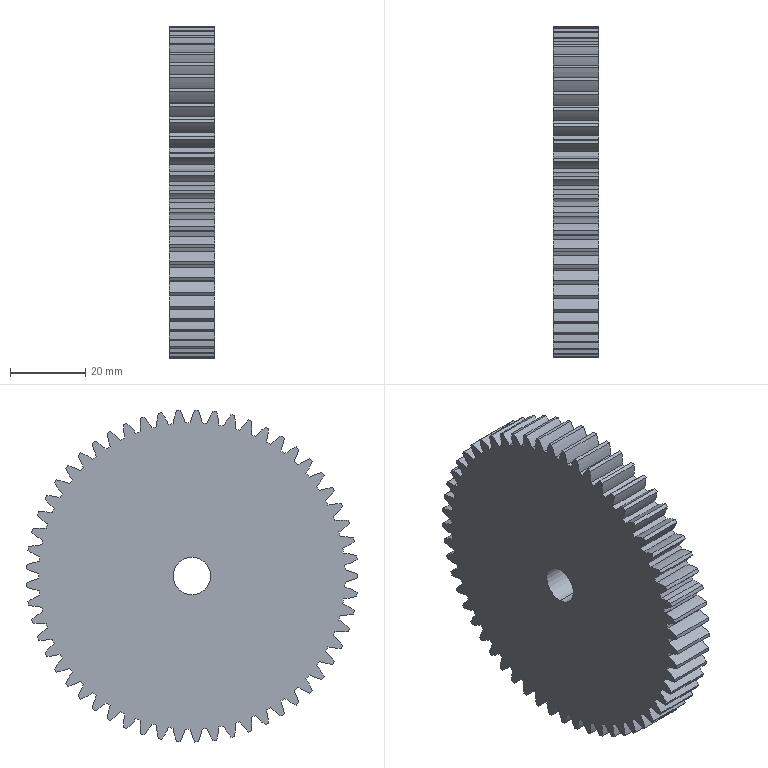Part | SolidWorks | features Boss 3, Cut 3, CirPattern 2, Fillet 2, Revolution 1 | 1 solid | 236 faces | box 12 x 88.457 x 88.488 mm | volume 67194 mm3 | cylinder 234 | plane 2 | commonest cylinder face diameters 34.2 x118 81.748 x57 88.5 x57 10 x2